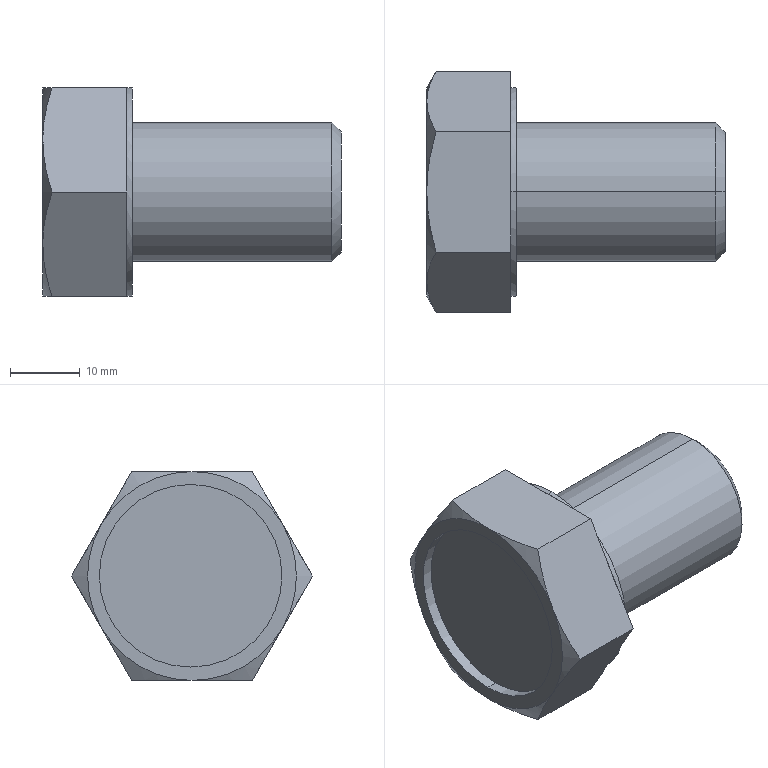Part | STEP file | formed hex screw_am_B18.2.3.2M - Formed hex screw, M20 x 2.5 x 30 --30WN | 1 solid | 30 faces | box 42.88 x 34.641 x 30 mm | volume 18448 mm3 | plane 16 | cone 8 | cylinder 6 | commonest cylinder face diameters 20 x2 26.25 x2 30 x2